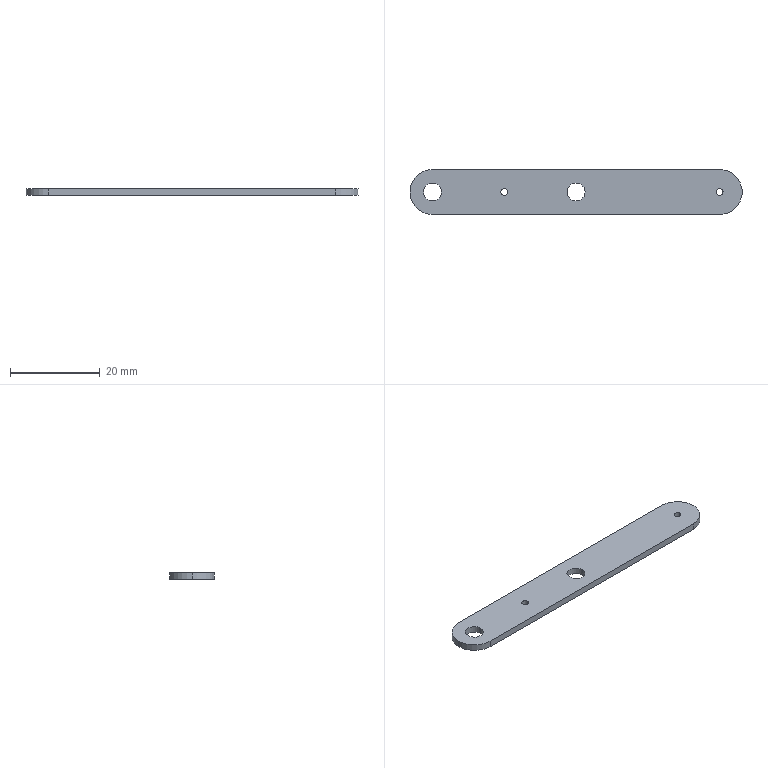Part | SolidWorks | features Extrusion 1 | 1 solid | 15 faces | box 74 x 10 x 1.5 mm | volume 1035 mm3 | cylinder 11 | plane 4 | commonest cylinder face diameters 1.5 x4 4 x4 10 x3
STEP:
#1=CARTESIAN_POINT('',(-27.299,0.,1.5));
#2=VERTEX_POINT('',#1);
#3=CARTESIAN_POINT('',(-23.299,0.,1.5));
#4=VERTEX_POINT('',#3);
#5=CARTESIAN_POINT('',(-25.299,0.,1.5));
#6=DIRECTION('',(0.,0.,1.));
#7=DIRECTION('',(1.,0.,0.));
#8=AXIS2_PLACEMENT_3D('',#5,#6,#7);
#9=CIRCLE('',#8,2.);
#10=EDGE_CURVE('',#2,#4,#9,.T.);
#11=ORIENTED_EDGE('',*,*,#10,.T.);
#12=CARTESIAN_POINT('',(-23.299,0.,0.));
#13=VERTEX_POINT('',#12);
#14=CARTESIAN_POINT('',(-23.299,0.,1.5));
#15=DIRECTION('',(0.,0.,-1.));
#16=VECTOR('',#15,1000.);
#17=LINE('',#14,#16);
#18=EDGE_CURVE('',#4,#13,#17,.T.);
#19=ORIENTED_EDGE('',*,*,#18,.T.);
#20=CARTESIAN_POINT('',(-27.299,0.,0.));
#21=VERTEX_POINT('',#20);
#22=CARTESIAN_POINT('',(-25.299,0.,0.));
#23=DIRECTION('',(0.,0.,1.));
#24=DIRECTION('',(1.,0.,0.));
#25=AXIS2_PLACEMENT_3D('',#22,#23,#24);
#26=CIRCLE('',#25,2.);
#27=EDGE_CURVE('',#21,#13,#26,.T.);
#28=ORIENTED_EDGE('',*,*,#27,.F.);
#29=CARTESIAN_POINT('',(-27.299,0.,1.5));
#30=DIRECTION('',(0.,0.,-1.));
#31=VECTOR('',#30,1000.);
#32=LINE('',#29,#31);
#33=EDGE_CURVE('',#2,#21,#32,.T.);
#34=ORIENTED_EDGE('',*,*,#33,.F.);
#35=EDGE_LOOP('',(#11,#19,#28,#34));
#36=FACE_OUTER_BOUND('',#35,.T.);
#37=CARTESIAN_POINT('',(-25.299,0.,1.5));
#38=DIRECTION('',(0.,0.,-1.));
#39=DIRECTION('',(-1.,0.,0.));
#40=AXIS2_PLACEMENT_3D('',#37,#38,#39);
#41=CYLINDRICAL_SURFACE('',#40,2.);
#42=ADVANCED_FACE('',(#36),#41,.F.);
#43=CARTESIAN_POINT('',(-42.049,0.,1.5));
#44=VERTEX_POINT('',#43);
#45=CARTESIAN_POINT('',(-40.549,0.,1.5));
#46=VERTEX_POINT('',#45);
#47=CARTESIAN_POINT('',(-41.299,0.,1.5));
#48=DIRECTION('',(0.,0.,1.));
#49=DIRECTION('',(1.,0.,0.));
#50=AXIS2_PLACEMENT_3D('',#47,#48,#49);
#51=CIRCLE('',#50,0.75);
#52=EDGE_CURVE('',#44,#46,#51,.T.);
#53=ORIENTED_EDGE('',*,*,#52,.T.);
#54=CARTESIAN_POINT('',(-40.549,0.,0.));
#55=VERTEX_POINT('',#54);
#56=CARTESIAN_POINT('',(-40.549,0.,1.5));
#57=DIRECTION('',(0.,0.,-1.));
#58=VECTOR('',#57,1000.);
#59=LINE('',#56,#58);
#60=EDGE_CURVE('',#46,#55,#59,.T.);
#61=ORIENTED_EDGE('',*,*,#60,.T.);
#62=CARTESIAN_POINT('',(-42.049,0.,0.));
#63=VERTEX_POINT('',#62);
#64=CARTESIAN_POINT('',(-41.299,0.,0.));
#65=DIRECTION('',(0.,0.,1.));
#66=DIRECTION('',(1.,0.,0.));
#67=AXIS2_PLACEMENT_3D('',#64,#65,#66);
#68=CIRCLE('',#67,0.75);
#69=EDGE_CURVE('',#63,#55,#68,.T.);
#70=ORIENTED_EDGE('',*,*,#69,.F.);
#71=CARTESIAN_POINT('',(-42.049,0.,1.5));
#72=DIRECTION('',(0.,0.,-1.));
#73=VECTOR('',#72,1000.);
#74=LINE('',#71,#73);
#75=EDGE_CURVE('',#44,#63,#74,.T.);
#76=ORIENTED_EDGE('',*,*,#75,.F.);
#77=EDGE_LOOP('',(#53,#61,#70,#76));
#78=FACE_OUTER_BOUND('',#77,.T.);
#79=CARTESIAN_POINT('',(-41.299,0.,1.5));
#80=DIRECTION('',(0.,0.,-1.));
#81=DIRECTION('',(-1.,0.,0.));
#82=AXIS2_PLACEMENT_3D('',#79,#80,#81);
#83=CYLINDRICAL_SURFACE('',#82,0.75);
#84=ADVANCED_FACE('',(#78),#83,.F.);
#85=CARTESIAN_POINT('',(5.951,0.,1.5));
#86=VERTEX_POINT('',#85);
#87=CARTESIAN_POINT('',(7.451,0.,1.5));
#88=VERTEX_POINT('',#87);
#89=CARTESIAN_POINT('',(6.701,0.,1.5));
#90=DIRECTION('',(0.,0.,1.));
#91=DIRECTION('',(1.,0.,0.));
#92=AXIS2_PLACEMENT_3D('',#89,#90,#91);
#93=CIRCLE('',#92,0.75);
#94=EDGE_CURVE('',#86,#88,#93,.T.);
#95=ORIENTED_EDGE('',*,*,#94,.T.);
#96=CARTESIAN_POINT('',(7.451,0.,0.));
#97=VERTEX_POINT('',#96);
#98=CARTESIAN_POINT('',(7.451,0.,1.5));
#99=DIRECTION('',(0.,0.,-1.));
#100=VECTOR('',#99,1000.);
#101=LINE('',#98,#100);
#102=EDGE_CURVE('',#88,#97,#101,.T.);
#103=ORIENTED_EDGE('',*,*,#102,.T.);
#104=CARTESIAN_POINT('',(5.951,0.,0.));
#105=VERTEX_POINT('',#104);
#106=CARTESIAN_POINT('',(6.701,0.,0.));
#107=DIRECTION('',(0.,0.,1.));
#108=DIRECTION('',(1.,0.,0.));
#109=AXIS2_PLACEMENT_3D('',#106,#107,#108);
#110=CIRCLE('',#109,0.75);
#111=EDGE_CURVE('',#105,#97,#110,.T.);
#112=ORIENTED_EDGE('',*,*,#111,.F.);
#113=CARTESIAN_POINT('',(5.951,0.,1.5));
#114=DIRECTION('',(0.,0.,-1.));
#115=VECTOR('',#114,1000.);
#116=LINE('',#113,#115);
#117=EDGE_CURVE('',#86,#105,#116,.T.);
#118=ORIENTED_EDGE('',*,*,#117,.F.);
#119=EDGE_LOOP('',(#95,#103,#112,#118));
#120=FACE_OUTER_BOUND('',#119,.T.);
#121=CARTESIAN_POINT('',(6.701,0.,1.5));
#122=DIRECTION('',(0.,0.,-1.));
#123=DIRECTION('',(-1.,0.,0.));
#124=AXIS2_PLACEMENT_3D('',#121,#122,#123);
#125=CYLINDRICAL_SURFACE('',#124,0.75);
#126=ADVANCED_FACE('',(#120),#125,.F.);
#127=CARTESIAN_POINT('',(-59.299,0.,1.5));
#128=VERTEX_POINT('',#127);
#129=CARTESIAN_POINT('',(-55.299,0.,1.5));
#130=VERTEX_POINT('',#129);
#131=CARTESIAN_POINT('',(-57.299,0.,1.5));
#132=DIRECTION('',(0.,0.,1.));
#133=DIRECTION('',(1.,0.,0.));
#134=AXIS2_PLACEMENT_3D('',#131,#132,#133);
#135=CIRCLE('',#134,2.);
#136=EDGE_CURVE('',#128,#130,#135,.T.);
#137=ORIENTED_EDGE('',*,*,#136,.T.);
#138=CARTESIAN_POINT('',(-55.299,0.,0.));
#139=VERTEX_POINT('',#138);
#140=CARTESIAN_POINT('',(-55.299,0.,1.5));
#141=DIRECTION('',(0.,0.,-1.));
#142=VECTOR('',#141,1000.);
#143=LINE('',#140,#142);
#144=EDGE_CURVE('',#130,#139,#143,.T.);
#145=ORIENTED_EDGE('',*,*,#144,.T.);
#146=CARTESIAN_POINT('',(-59.299,0.,0.));
#147=VERTEX_POINT('',#146);
#148=CARTESIAN_POINT('',(-57.299,0.,0.));
#149=DIRECTION('',(0.,0.,1.));
#150=DIRECTION('',(1.,0.,0.));
#151=AXIS2_PLACEMENT_3D('',#148,#149,#150);
#152=CIRCLE('',#151,2.);
#153=EDGE_CURVE('',#147,#139,#152,.T.);
#154=ORIENTED_EDGE('',*,*,#153,.F.);
#155=CARTESIAN_POINT('',(-59.299,0.,1.5));
#156=DIRECTION('',(0.,0.,-1.));
#157=VECTOR('',#156,1000.);
#158=LINE('',#155,#157);
#159=EDGE_CURVE('',#128,#147,#158,.T.);
#160=ORIENTED_EDGE('',*,*,#159,.F.);
#161=EDGE_LOOP('',(#137,#145,#154,#160));
#162=FACE_OUTER_BOUND('',#161,.T.);
#163=CARTESIAN_POINT('',(-57.299,0.,1.5));
#164=DIRECTION('',(0.,0.,-1.));
#165=DIRECTION('',(-1.,0.,0.));
#166=AXIS2_PLACEMENT_3D('',#163,#164,#165);
#167=CYLINDRICAL_SURFACE('',#166,2.);
#168=ADVANCED_FACE('',(#162),#167,.F.);
#169=CARTESIAN_POINT('',(-62.299,0.,1.5));
#170=VERTEX_POINT('',#169);
#171=CARTESIAN_POINT('',(-57.299,-5.,1.5));
#172=VERTEX_POINT('',#171);
#173=CARTESIAN_POINT('',(-57.299,0.,1.5));
#174=DIRECTION('',(0.,0.,1.));
#175=DIRECTION('',(1.,0.,0.));
#176=AXIS2_PLACEMENT_3D('',#173,#174,#175);
#177=CIRCLE('',#176,5.);
#178=EDGE_CURVE('',#170,#172,#177,.T.);
#179=ORIENTED_EDGE('',*,*,#178,.F.);
#180=CARTESIAN_POINT('',(-62.299,0.,0.));
#181=VERTEX_POINT('',#180);
#182=CARTESIAN_POINT('',(-62.299,0.,1.5));
#183=DIRECTION('',(0.,0.,-1.));
#184=VECTOR('',#183,1000.);
#185=LINE('',#182,#184);
#186=EDGE_CURVE('',#170,#181,#185,.T.);
#187=ORIENTED_EDGE('',*,*,#186,.T.);
#188=CARTESIAN_POINT('',(-57.299,-5.,0.));
#189=VERTEX_POINT('',#188);
#190=CARTESIAN_POINT('',(-57.299,0.,0.));
#191=DIRECTION('',(0.,0.,1.));
#192=DIRECTION('',(1.,0.,0.));
#193=AXIS2_PLACEMENT_3D('',#190,#191,#192);
#194=CIRCLE('',#193,5.);
#195=EDGE_CURVE('',#181,#189,#194,.T.);
#196=ORIENTED_EDGE('',*,*,#195,.T.);
#197=CARTESIAN_POINT('',(-57.299,-5.,1.5));
#198=DIRECTION('',(0.,0.,-1.));
#199=VECTOR('',#198,1000.);
#200=LINE('',#197,#199);
#201=EDGE_CURVE('',#172,#189,#200,.T.);
#202=ORIENTED_EDGE('',*,*,#201,.F.);
#203=EDGE_LOOP('',(#179,#187,#196,#202));
#204=FACE_OUTER_BOUND('',#203,.T.);
#205=CARTESIAN_POINT('',(-57.299,0.,1.5));
#206=DIRECTION('',(0.,0.,-1.));
#207=DIRECTION('',(-1.,0.,0.));
#208=AXIS2_PLACEMENT_3D('',#205,#206,#207);
#209=CYLINDRICAL_SURFACE('',#208,5.);
#210=ADVANCED_FACE('',(#204),#209,.T.);
#211=ORIENTED_EDGE('',*,*,#52,.F.);
#212=CARTESIAN_POINT('',(-41.299,0.,1.5));
#213=DIRECTION('',(0.,0.,1.));
#214=DIRECTION('',(1.,0.,0.));
#215=AXIS2_PLACEMENT_3D('',#212,#213,#214);
#216=CIRCLE('',#215,0.75);
#217=EDGE_CURVE('',#46,#44,#216,.T.);
#218=ORIENTED_EDGE('',*,*,#217,.F.);
#219=EDGE_LOOP('',(#211,#218));
#220=FACE_BOUND('',#219,.T.);
#221=ORIENTED_EDGE('',*,*,#136,.F.);
#222=CARTESIAN_POINT('',(-57.299,0.,1.5));
#223=DIRECTION('',(0.,0.,1.));
#224=DIRECTION('',(1.,0.,0.));
#225=AXIS2_PLACEMENT_3D('',#222,#223,#224);
#226=CIRCLE('',#225,2.);
#227=EDGE_CURVE('',#130,#128,#226,.T.);
#228=ORIENTED_EDGE('',*,*,#227,.F.);
#229=EDGE_LOOP('',(#221,#228));
#230=FACE_BOUND('',#229,.T.);
#231=CARTESIAN_POINT('',(-57.299,5.,1.5));
#232=VERTEX_POINT('',#231);
#233=CARTESIAN_POINT('',(-57.299,0.,1.5));
#234=DIRECTION('',(0.,0.,1.));
#235=DIRECTION('',(1.,0.,0.));
#236=AXIS2_PLACEMENT_3D('',#233,#234,#235);
#237=CIRCLE('',#236,5.);
#238=EDGE_CURVE('',#232,#170,#237,.T.);
#239=ORIENTED_EDGE('',*,*,#238,.T.);
#240=ORIENTED_EDGE('',*,*,#178,.T.);
#241=CARTESIAN_POINT('',(6.701,-5.,1.5));
#242=VERTEX_POINT('',#241);
#243=CARTESIAN_POINT('',(-57.299,-5.,1.5));
#244=DIRECTION('',(1.,0.,0.));
#245=VECTOR('',#244,1000.);
#246=LINE('',#243,#245);
#247=EDGE_CURVE('',#172,#242,#246,.T.);
#248=ORIENTED_EDGE('',*,*,#247,.T.);
#249=CARTESIAN_POINT('',(6.701,5.,1.5));
#250=VERTEX_POINT('',#249);
#251=CARTESIAN_POINT('',(6.701,0.,1.5));
#252=DIRECTION('',(0.,0.,1.));
#253=DIRECTION('',(1.,0.,0.));
#254=AXIS2_PLACEMENT_3D('',#251,#252,#253);
#255=CIRCLE('',#254,5.);
#256=EDGE_CURVE('',#242,#250,#255,.T.);
#257=ORIENTED_EDGE('',*,*,#256,.T.);
#258=CARTESIAN_POINT('',(-57.299,5.,1.5));
#259=DIRECTION('',(-1.,0.,0.));
#260=VECTOR('',#259,1000.);
#261=LINE('',#258,#260);
#262=EDGE_CURVE('',#250,#232,#261,.T.);
#263=ORIENTED_EDGE('',*,*,#262,.T.);
#264=EDGE_LOOP('',(#239,#240,#248,#257,#263));
#265=FACE_OUTER_BOUND('',#264,.T.);
#266=ORIENTED_EDGE('',*,*,#94,.F.);
#267=CARTESIAN_POINT('',(6.701,0.,1.5));
#268=DIRECTION('',(0.,0.,1.));
#269=DIRECTION('',(1.,0.,0.));
#270=AXIS2_PLACEMENT_3D('',#267,#268,#269);
#271=CIRCLE('',#270,0.75);
#272=EDGE_CURVE('',#88,#86,#271,.T.);
#273=ORIENTED_EDGE('',*,*,#272,.F.);
#274=EDGE_LOOP('',(#266,#273));
#275=FACE_BOUND('',#274,.T.);
#276=ORIENTED_EDGE('',*,*,#10,.F.);
#277=CARTESIAN_POINT('',(-25.299,0.,1.5));
#278=DIRECTION('',(0.,0.,1.));
#279=DIRECTION('',(1.,0.,0.));
#280=AXIS2_PLACEMENT_3D('',#277,#278,#279);
#281=CIRCLE('',#280,2.);
#282=EDGE_CURVE('',#4,#2,#281,.T.);
#283=ORIENTED_EDGE('',*,*,#282,.F.);
#284=EDGE_LOOP('',(#276,#283));
#285=FACE_BOUND('',#284,.T.);
#286=CARTESIAN_POINT('',(-57.299,0.,1.5));
#287=DIRECTION('',(0.,0.,1.));
#288=DIRECTION('',(1.,0.,0.));
#289=AXIS2_PLACEMENT_3D('',#286,#287,#288);
#290=PLANE('',#289);
#291=ADVANCED_FACE('',(#220,#230,#265,#275,#285),#290,.T.);
#292=CARTESIAN_POINT('',(-57.299,5.,0.));
#293=VERTEX_POINT('',#292);
#294=CARTESIAN_POINT('',(-57.299,0.,0.));
#295=DIRECTION('',(0.,0.,1.));
#296=DIRECTION('',(1.,0.,0.));
#297=AXIS2_PLACEMENT_3D('',#294,#295,#296);
#298=CIRCLE('',#297,5.);
#299=EDGE_CURVE('',#293,#181,#298,.T.);
#300=ORIENTED_EDGE('',*,*,#299,.F.);
#301=CARTESIAN_POINT('',(6.701,5.,0.));
#302=VERTEX_POINT('',#301);
#303=CARTESIAN_POINT('',(-57.299,5.,0.));
#304=DIRECTION('',(-1.,0.,0.));
#305=VECTOR('',#304,1000.);
#306=LINE('',#303,#305);
#307=EDGE_CURVE('',#302,#293,#306,.T.);
#308=ORIENTED_EDGE('',*,*,#307,.F.);
#309=CARTESIAN_POINT('',(6.701,-5.,0.));
#310=VERTEX_POINT('',#309);
#311=CARTESIAN_POINT('',(6.701,0.,0.));
#312=DIRECTION('',(0.,0.,1.));
#313=DIRECTION('',(1.,0.,0.));
#314=AXIS2_PLACEMENT_3D('',#311,#312,#313);
#315=CIRCLE('',#314,5.);
#316=EDGE_CURVE('',#310,#302,#315,.T.);
#317=ORIENTED_EDGE('',*,*,#316,.F.);
#318=CARTESIAN_POINT('',(-57.299,-5.,0.));
#319=DIRECTION('',(1.,0.,0.));
#320=VECTOR('',#319,1000.);
#321=LINE('',#318,#320);
#322=EDGE_CURVE('',#189,#310,#321,.T.);
#323=ORIENTED_EDGE('',*,*,#322,.F.);
#324=ORIENTED_EDGE('',*,*,#195,.F.);
#325=EDGE_LOOP('',(#300,#308,#317,#323,#324));
#326=FACE_OUTER_BOUND('',#325,.T.);
#327=ORIENTED_EDGE('',*,*,#153,.T.);
#328=CARTESIAN_POINT('',(-57.299,0.,0.));
#329=DIRECTION('',(0.,0.,1.));
#330=DIRECTION('',(1.,0.,0.));
#331=AXIS2_PLACEMENT_3D('',#328,#329,#330);
#332=CIRCLE('',#331,2.);
#333=EDGE_CURVE('',#139,#147,#332,.T.);
#334=ORIENTED_EDGE('',*,*,#333,.T.);
#335=EDGE_LOOP('',(#327,#334));
#336=FACE_BOUND('',#335,.T.);
#337=ORIENTED_EDGE('',*,*,#111,.T.);
#338=CARTESIAN_POINT('',(6.701,0.,0.));
#339=DIRECTION('',(0.,0.,1.));
#340=DIRECTION('',(1.,0.,0.));
#341=AXIS2_PLACEMENT_3D('',#338,#339,#340);
#342=CIRCLE('',#341,0.75);
#343=EDGE_CURVE('',#97,#105,#342,.T.);
#344=ORIENTED_EDGE('',*,*,#343,.T.);
#345=EDGE_LOOP('',(#337,#344));
#346=FACE_BOUND('',#345,.T.);
#347=ORIENTED_EDGE('',*,*,#69,.T.);
#348=CARTESIAN_POINT('',(-41.299,0.,0.));
#349=DIRECTION('',(0.,0.,1.));
#350=DIRECTION('',(1.,0.,0.));
#351=AXIS2_PLACEMENT_3D('',#348,#349,#350);
#352=CIRCLE('',#351,0.75);
#353=EDGE_CURVE('',#55,#63,#352,.T.);
#354=ORIENTED_EDGE('',*,*,#353,.T.);
#355=EDGE_LOOP('',(#347,#354));
#356=FACE_BOUND('',#355,.T.);
#357=ORIENTED_EDGE('',*,*,#27,.T.);
#358=CARTESIAN_POINT('',(-25.299,0.,0.));
#359=DIRECTION('',(0.,0.,1.));
#360=DIRECTION('',(1.,0.,0.));
#361=AXIS2_PLACEMENT_3D('',#358,#359,#360);
#362=CIRCLE('',#361,2.);
#363=EDGE_CURVE('',#13,#21,#362,.T.);
#364=ORIENTED_EDGE('',*,*,#363,.T.);
#365=EDGE_LOOP('',(#357,#364));
#366=FACE_BOUND('',#365,.T.);
#367=CARTESIAN_POINT('',(-57.299,0.,0.));
#368=DIRECTION('',(0.,0.,1.));
#369=DIRECTION('',(1.,0.,0.));
#370=AXIS2_PLACEMENT_3D('',#367,#368,#369);
#371=PLANE('',#370);
#372=ADVANCED_FACE('',(#326,#336,#346,#356,#366),#371,.F.);
#373=ORIENTED_EDGE('',*,*,#186,.F.);
#374=ORIENTED_EDGE('',*,*,#238,.F.);
#375=CARTESIAN_POINT('',(-57.299,5.,1.5));
#376=DIRECTION('',(0.,0.,-1.));
#377=VECTOR('',#376,1000.);
#378=LINE('',#375,#377);
#379=EDGE_CURVE('',#232,#293,#378,.T.);
#380=ORIENTED_EDGE('',*,*,#379,.T.);
#381=ORIENTED_EDGE('',*,*,#299,.T.);
#382=EDGE_LOOP('',(#373,#374,#380,#381));
#383=FACE_OUTER_BOUND('',#382,.T.);
#384=CARTESIAN_POINT('',(-57.299,0.,1.5));
#385=DIRECTION('',(0.,0.,-1.));
#386=DIRECTION('',(-1.,0.,0.));
#387=AXIS2_PLACEMENT_3D('',#384,#385,#386);
#388=CYLINDRICAL_SURFACE('',#387,5.);
#389=ADVANCED_FACE('',(#383),#388,.T.);
#390=ORIENTED_EDGE('',*,*,#322,.T.);
#391=CARTESIAN_POINT('',(6.701,-5.,1.5));
#392=DIRECTION('',(0.,0.,-1.));
#393=VECTOR('',#392,1000.);
#394=LINE('',#391,#393);
#395=EDGE_CURVE('',#242,#310,#394,.T.);
#396=ORIENTED_EDGE('',*,*,#395,.F.);
#397=ORIENTED_EDGE('',*,*,#247,.F.);
#398=ORIENTED_EDGE('',*,*,#201,.T.);
#399=EDGE_LOOP('',(#390,#396,#397,#398));
#400=FACE_OUTER_BOUND('',#399,.T.);
#401=CARTESIAN_POINT('',(-57.299,-5.,1.5));
#402=DIRECTION('',(0.,1.,0.));
#403=DIRECTION('',(-1.,0.,0.));
#404=AXIS2_PLACEMENT_3D('',#401,#402,#403);
#405=PLANE('',#404);
#406=ADVANCED_FACE('',(#400),#405,.F.);
#407=ORIENTED_EDGE('',*,*,#316,.T.);
#408=CARTESIAN_POINT('',(6.701,5.,1.5));
#409=DIRECTION('',(0.,0.,-1.));
#410=VECTOR('',#409,1000.);
#411=LINE('',#408,#410);
#412=EDGE_CURVE('',#250,#302,#411,.T.);
#413=ORIENTED_EDGE('',*,*,#412,.F.);
#414=ORIENTED_EDGE('',*,*,#256,.F.);
#415=ORIENTED_EDGE('',*,*,#395,.T.);
#416=EDGE_LOOP('',(#407,#413,#414,#415));
#417=FACE_OUTER_BOUND('',#416,.T.);
#418=CARTESIAN_POINT('',(6.701,0.,1.5));
#419=DIRECTION('',(0.,0.,-1.));
#420=DIRECTION('',(-1.,0.,0.));
#421=AXIS2_PLACEMENT_3D('',#418,#419,#420);
#422=CYLINDRICAL_SURFACE('',#421,5.);
#423=ADVANCED_FACE('',(#417),#422,.T.);
#424=ORIENTED_EDGE('',*,*,#307,.T.);
#425=ORIENTED_EDGE('',*,*,#379,.F.);
#426=ORIENTED_EDGE('',*,*,#262,.F.);
#427=ORIENTED_EDGE('',*,*,#412,.T.);
#428=EDGE_LOOP('',(#424,#425,#426,#427));
#429=FACE_OUTER_BOUND('',#428,.T.);
#430=CARTESIAN_POINT('',(-57.299,5.,1.5));
#431=DIRECTION('',(0.,-1.,0.));
#432=DIRECTION('',(1.,0.,0.));
#433=AXIS2_PLACEMENT_3D('',#430,#431,#432);
#434=PLANE('',#433);
#435=ADVANCED_FACE('',(#429),#434,.F.);
#436=ORIENTED_EDGE('',*,*,#144,.F.);
#437=ORIENTED_EDGE('',*,*,#227,.T.);
#438=ORIENTED_EDGE('',*,*,#159,.T.);
#439=ORIENTED_EDGE('',*,*,#333,.F.);
#440=EDGE_LOOP('',(#436,#437,#438,#439));
#441=FACE_OUTER_BOUND('',#440,.T.);
#442=CARTESIAN_POINT('',(-57.299,0.,1.5));
#443=DIRECTION('',(0.,0.,-1.));
#444=DIRECTION('',(-1.,0.,0.));
#445=AXIS2_PLACEMENT_3D('',#442,#443,#444);
#446=CYLINDRICAL_SURFACE('',#445,2.);
#447=ADVANCED_FACE('',(#441),#446,.F.);
#448=ORIENTED_EDGE('',*,*,#102,.F.);
#449=ORIENTED_EDGE('',*,*,#272,.T.);
#450=ORIENTED_EDGE('',*,*,#117,.T.);
#451=ORIENTED_EDGE('',*,*,#343,.F.);
#452=EDGE_LOOP('',(#448,#449,#450,#451));
#453=FACE_OUTER_BOUND('',#452,.T.);
#454=CARTESIAN_POINT('',(6.701,0.,1.5));
#455=DIRECTION('',(0.,0.,-1.));
#456=DIRECTION('',(-1.,0.,0.));
#457=AXIS2_PLACEMENT_3D('',#454,#455,#456);
#458=CYLINDRICAL_SURFACE('',#457,0.75);
#459=ADVANCED_FACE('',(#453),#458,.F.);
#460=ORIENTED_EDGE('',*,*,#60,.F.);
#461=ORIENTED_EDGE('',*,*,#217,.T.);
#462=ORIENTED_EDGE('',*,*,#75,.T.);
#463=ORIENTED_EDGE('',*,*,#353,.F.);
#464=EDGE_LOOP('',(#460,#461,#462,#463));
#465=FACE_OUTER_BOUND('',#464,.T.);
#466=CARTESIAN_POINT('',(-41.299,0.,1.5));
#467=DIRECTION('',(0.,0.,-1.));
#468=DIRECTION('',(-1.,0.,0.));
#469=AXIS2_PLACEMENT_3D('',#466,#467,#468);
#470=CYLINDRICAL_SURFACE('',#469,0.75);
#471=ADVANCED_FACE('',(#465),#470,.F.);
#472=ORIENTED_EDGE('',*,*,#18,.F.);
#473=ORIENTED_EDGE('',*,*,#282,.T.);
#474=ORIENTED_EDGE('',*,*,#33,.T.);
#475=ORIENTED_EDGE('',*,*,#363,.F.);
#476=EDGE_LOOP('',(#472,#473,#474,#475));
#477=FACE_OUTER_BOUND('',#476,.T.);
#478=CARTESIAN_POINT('',(-25.299,0.,1.5));
#479=DIRECTION('',(0.,0.,-1.));
#480=DIRECTION('',(-1.,0.,0.));
#481=AXIS2_PLACEMENT_3D('',#478,#479,#480);
#482=CYLINDRICAL_SURFACE('',#481,2.);
#483=ADVANCED_FACE('',(#477),#482,.F.);
#484=CLOSED_SHELL('',(#42,#84,#126,#168,#210,#291,#372,#389,#406,#423,#435,#447,#459,#471,#483));
#485=MANIFOLD_SOLID_BREP('',#484);
#486=CARTESIAN_POINT('',(0.,0.,0.));
#487=DIRECTION('',(0.,0.,1.));
#488=DIRECTION('',(1.,0.,0.));
#489=AXIS2_PLACEMENT_3D('',#486,#487,#488);
#490=(LENGTH_UNIT()NAMED_UNIT(*)SI_UNIT(.MILLI.,.METRE.));
#491=UNCERTAINTY_MEASURE_WITH_UNIT(LENGTH_MEASURE(0.00001),#490,'','');
#492=(NAMED_UNIT(*)PLANE_ANGLE_UNIT()SI_UNIT($,.RADIAN.));
#493=(NAMED_UNIT(*)SI_UNIT($,.STERADIAN.)SOLID_ANGLE_UNIT());
#494=(GEOMETRIC_REPRESENTATION_CONTEXT(3)GLOBAL_UNCERTAINTY_ASSIGNED_CONTEXT((#491))GLOBAL_UNIT_ASSIGNED_CONTEXT((#490,#492,#493))REPRESENTATION_CONTEXT('',''));
#495=ADVANCED_BREP_SHAPE_REPRESENTATION('',(#485,#489),#494);